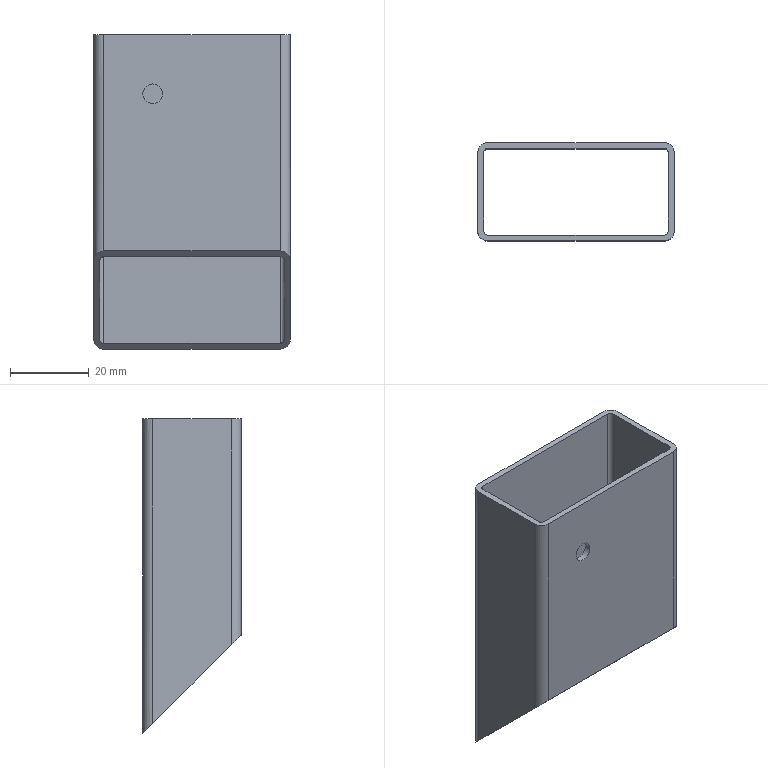Part | STEP file | 5091401L | 1 solid | 19 faces | box 50 x 25 x 80 mm | volume 14246 mm3 | plane 10 | cylinder 9 | commonest cylinder face diameters 5 x5 2 x4